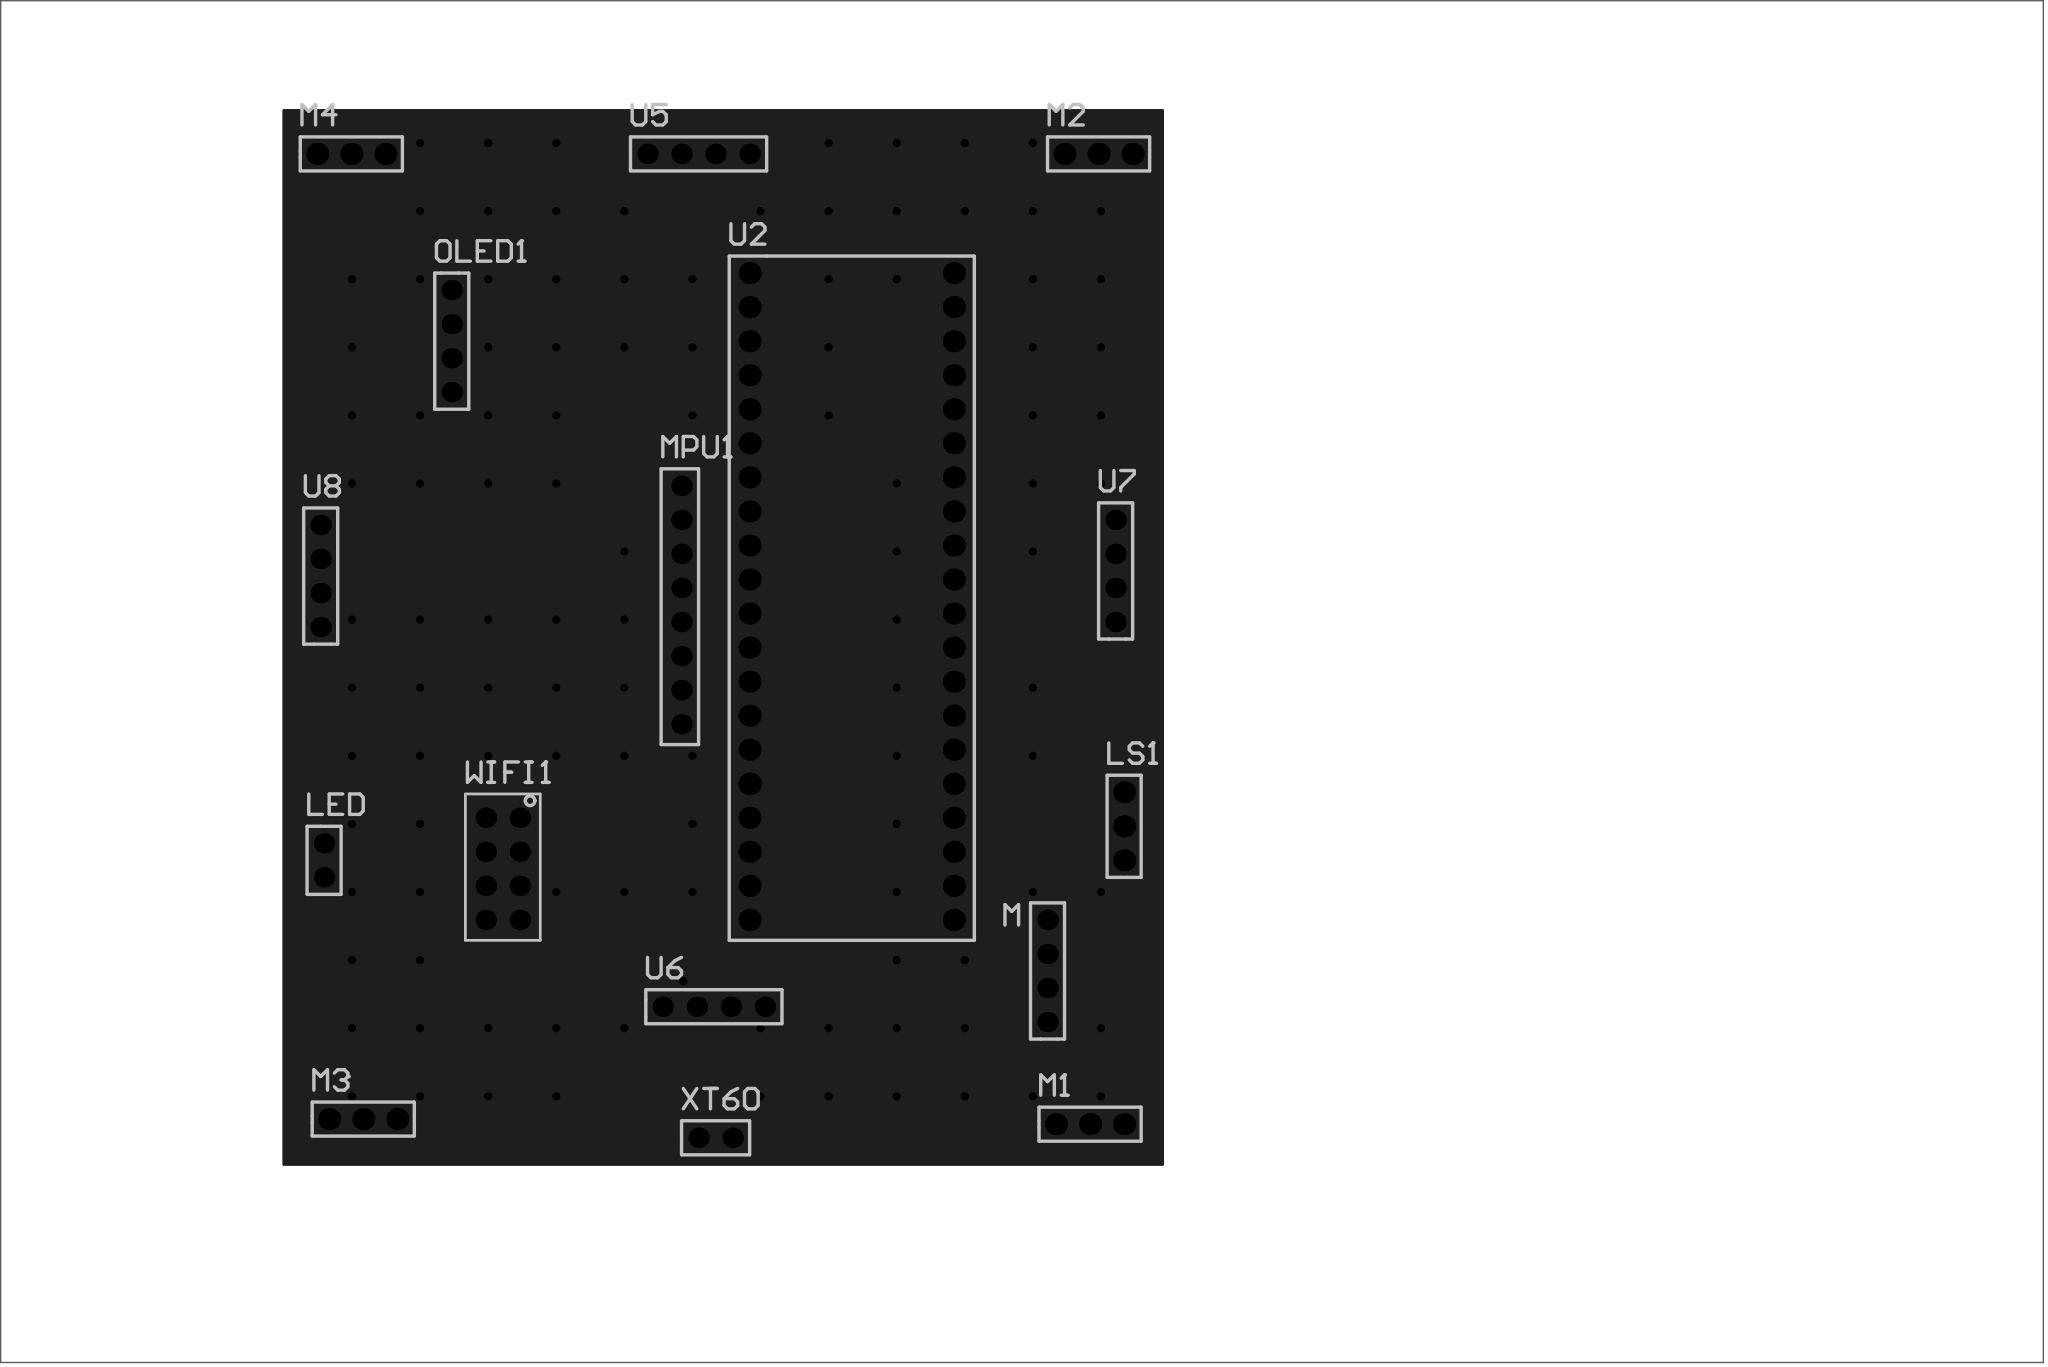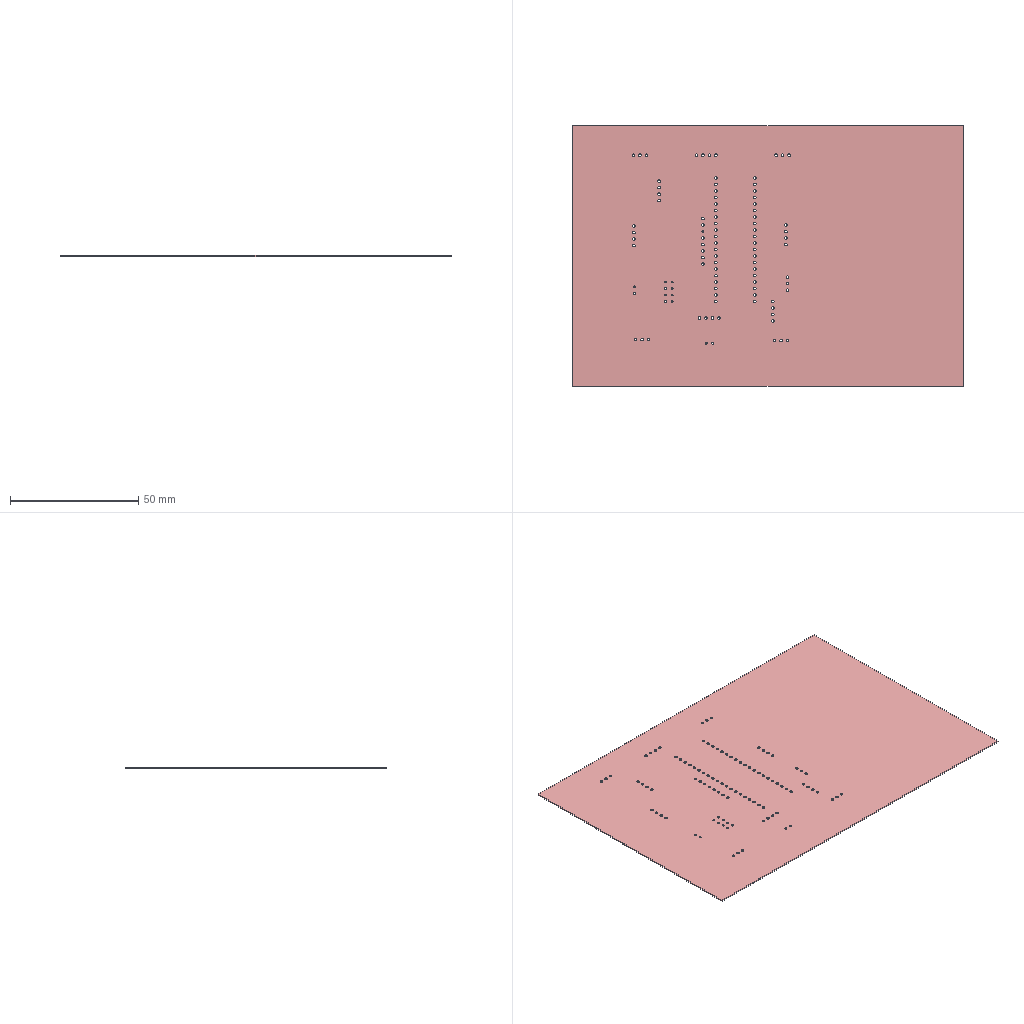Circuit board layout | Altium Designer | box 152.4 x 101.6 x 0.4 mm
Layer stack:
# Altium Designer layer stack of  (unit mm; dielectric type: 0 none, 1 core, 2 prepreg, 3 surface material)
index,name,kind,layer,copper_thickness_mm,dielectric_type,dielectric_thickness_mm,dielectric_material,dielectric_constant
0,Top Paste Mask Layer,other,,,,,,
1,Top Silkscreen Layer,other,,,,,,
2,Top Solder Mask Layer,dielectric,,,3,0.0102,Solder Resist,3.5
3,Top Layer,copper,Top Layer,0.0356,,,,
4,Dielectric 1,dielectric,,,3,0.32,FR-4,4.8
5,Bottom Layer,copper,Bottom Layer,0.0356,,,,
6,Bottom Solder Mask Layer,dielectric,,,3,0.0102,Solder Resist,3.5
7,Bottom Silkscreen Layer,other,,,,,,
8,Bottom Paste Mask Layer,other,,,,,,
# drill layer pairs: low layer,high layer
drill_pair,Top Layer,Bottom Layer
Part placement:
Designator,Comment,Layer,Footprint,Center-X(mm),Center-Y(mm),Rotation
M,MH-SENSOR,TopLayer,OLED,154.305,105.41,180
LED,LED,TopLayer,XT60,100.33,113.665,0
U8,HC-SR04,TopLayer,OLED,100.076,134.874,180
U7,HC-SR04,TopLayer,OLED,159.385,135.255,180
U6,HC-SR04,TopLayer,OLED,129.413,102.743,90
WIFI1,ESP8266,TopLayer,ESP8266,113.665,113.03,270
U5,HC-SR04,TopLayer,OLED,128.27,166.37,90
U2,STM32_BluePill,TopLayer,STM32_BluePill_1,139.7,133.35,0
XT60,XT60,TopLayer,XT60,129.54,92.964,90
OLED1,OLED,TopLayer,OLED,109.855,152.4,0
MPU1,MPU6050,TopLayer,MPU6050,127,132.715,0
M4,header_3,TopLayer,header,102.362,166.37,90
M3,header_3,TopLayer,header,103.251,94.361,90
M2,header_3,TopLayer,header,158.115,166.37,270
M1,header_3,TopLayer,header,157.48,93.98,90
LS1,Buzzer,TopLayer,header,160.02,116.205,180
Pad and via stacks:
# Altium Designer via and pad stacks of  (unit mm). Each distinct definition once, with the count of objects using it.
# via: kind,start_layer,end_layer,hole_mm,diameter_mm,mode(0 simple;1 top-mid-bottom;2 full stack),diameter_per_layer,count,example_net
# pad: kind,layer,hole_mm,hole_type(0 round;1 square;2 slot),plating,top_size,top_shape(1 round;2 rect;3 octagon;9 rounded rect),mid_size,bottom_size,mode,footprint,size_per_layer,count,example
pad,Multi-Layer,1.016,0,plated,1.524x1.524,1,1.524x1.524,1.524x1.524,0,OLED,,24,M.1
pad,Multi-Layer,0.762,0,plated,1.524x1.524,1,1.524x1.524,1.524x1.524,0,XT60,,4,LED.1
pad,Multi-Layer,0.762,0,plated,1.524x1.524,1,1.524x1.524,1.524x1.524,0,ESP8266,,8,WIFI1.5
pad,Multi-Layer,1.016,0,plated,1.651x1.651,1,1.651x1.651,1.651x1.651,0,STM32_BluePill_1,,41,U2.1
pad,Multi-Layer,1.016,0,plated,1.524x1.524,1,1.524x1.524,1.524x1.524,0,MPU6050,,7,MPU1.8
pad,Multi-Layer,0.762,0,plated,1.524x1.524,1,1.524x1.524,1.524x1.524,0,MPU6050,,1,MPU1.3
pad,Multi-Layer,1.016,0,plated,1.651x1.651,1,1.651x1.651,1.651x1.651,0,header,,15,M4.3
via,Top Layer,Bottom Layer,0.3048,0.61,0,,1,Echo_B
via,Top Layer,Bottom Layer,0.3048,0.6096,0,,110,GND
Copper pours:
name,layer,net,type(0 solid;1 hatched;2 none)
Top Layer-GND,Top Layer,GND,0
Bottom Layer-GND,Bottom Layer,GND,0
Design rules, without the lines most boards share:
# Altium Designer design rules of  (exported by Altium Designer, unit mm)
# columns: name | kind | enabled | priority | scope1 | scope2 | descriptor | typed fields (field=value)
ComponentClearance_1 | 24 | enabled | 1 | All | All | Component Clearance Constraint ( Horizontal Gap = 10mil, Vertical Gap = 10mil ) (All),(All)  | gap=0.254
Clearance | 0 | enabled | 1 | All | All | Clearance Constraint (Gap=7.874mil) (All),(All) | gap=0.2
Clearance_1 | 63 | enabled | 1 | All | All | Board Clearance Constraint (Gap=0mil) (All) |
creepage | 65 | enabled | 1 | All | All | Creepage Distance Constraint =(0mil) (All),(All) |
ComponentClearance | 52 | enabled | 1 | All | All | Hole To Hole Clearance (Gap=10mil) (All),(All) | gap=0.254
Power_Path | 2 | enabled | 1 | (InNet('3.3V') OR InNet('+5') OR InNet('GND')) | All | Width Constraint (Min=15mil) (Max=25.6mil) (Preferred=25.6mil) ((InNet('3.3V') OR InNet('+5') OR InNet('GND'))) |
Width | 2 | enabled | 2 | All | All | Width Constraint (Min=5.9mil) (Max=23.6mil) (Preferred=7.9mil) (All) |
DiffPairsRouting | 51 | enabled | 1 | All | All | Differential Pairs Uncoupled Length using the Gap Constraints (Min=10mil) (Max=10mil) (Prefered=10mil)  and Width Constraints (Min=15mil) (Max=15mil) (Prefered=15mil) (All) |
RoutingVias | 11 | enabled | 1 | All | All | Routing Via (MinHoleWidth=1mil) (MaxHoleWidth=28mil) (PreferredHoleWidth=28mil) (MinWidth=1mil) (MaxWidth=50mil) (PreferedWidth=50mil) (All) | via_min_hole=0.0254 via_max_hole=0.7112 via_preferred_diameter=1.27 via_preferred_hole=0.7112
PlaneConnect | 6 | enabled | 1 | All | All | Power Plane Connect Rule(Relief Connect )(Expansion=20mil) (Conductor Width=10mil) (Air Gap=10mil) (Entries=4) (All) | relief_conductor_width=0.254 relief_entries=4 relief_expansion=0.508
PolygonConnect | 20 | enabled | 1 | (InNet('GND')) | All | Polygon Connect Rule(Relief Connect )(Conductor Width=10mil) (Relief Angle=90 Angle) (Entries=4) (Air Gap Width=10mil) ((InNet('GND'))),(All) | connect_style(0=relief,1=direct,2=none)=0 relief_conductor_width=0.254 relief_entries=4
PasteMaskExpansion | 14 | enabled | 1 | All | All | Paste Mask Expansion (Expansion =0mil) (All) | expansion=0
SolderMaskExpansion | 13 | enabled | 1 | All | All | Solder Mask Expansion (Expansion =4mil) (All) | expansion=0.1016